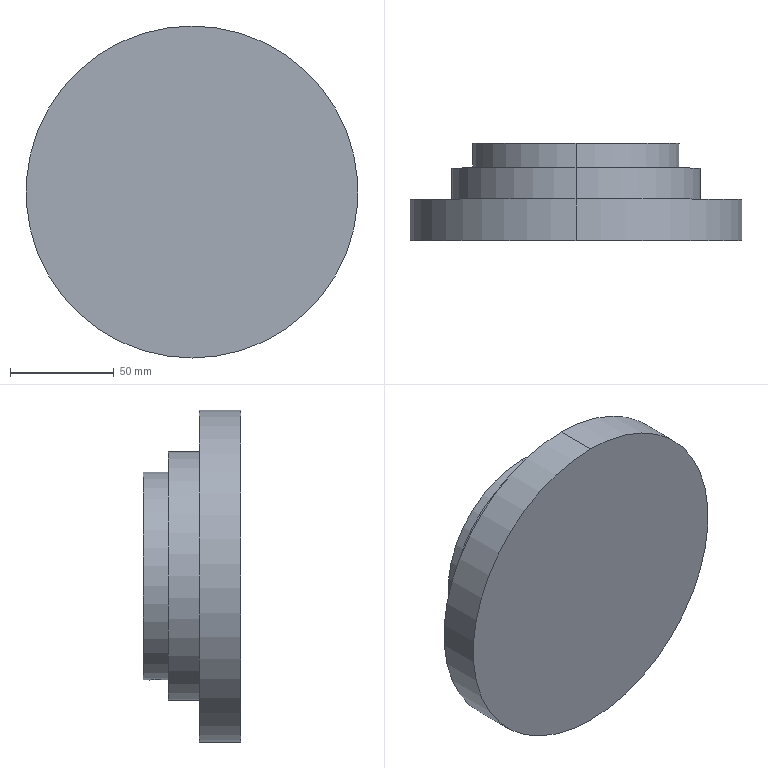Part | SolidWorks | features ICE 4, HoleWzd 2, 3DProfileFeature 1, Extrusion 1, SweepThread 1 | 1 solid | 66 faces | box 160 x 47 x 160 mm | volume 641630 mm3 | cylinder 54 | plane 8 | spline 4 | commonest cylinder face diameters 6.8 x44 8 x2 50 x2 100 x2 120 x2 160 x2